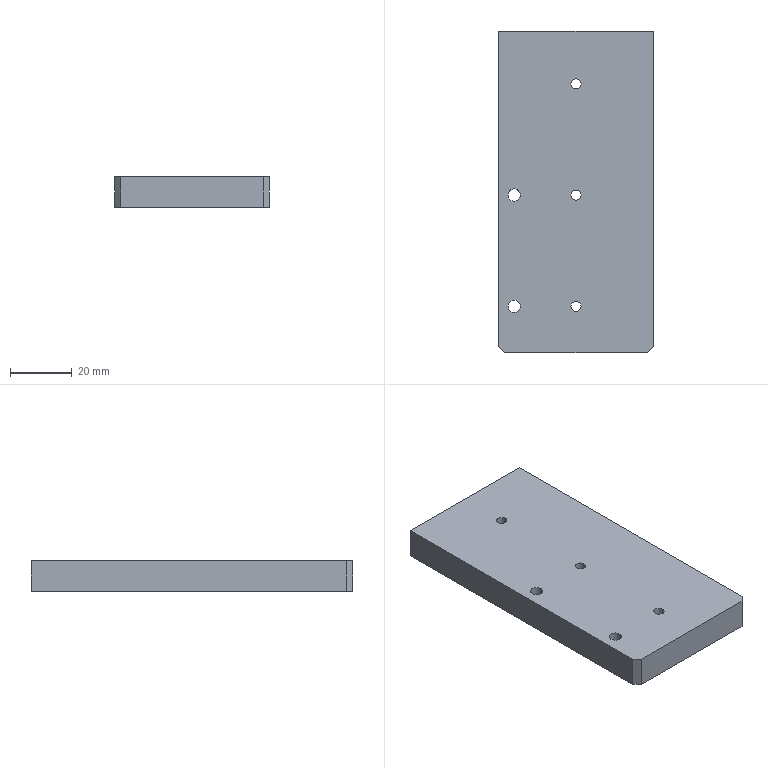Part | STEP file | QA-FB10 | 1 solid | 38 faces | box 50 x 104 x 10 mm | volume 50937 mm3 | cylinder 20 | cone 10 | plane 8 | commonest cylinder face diameters 3.3 x12 4 x8